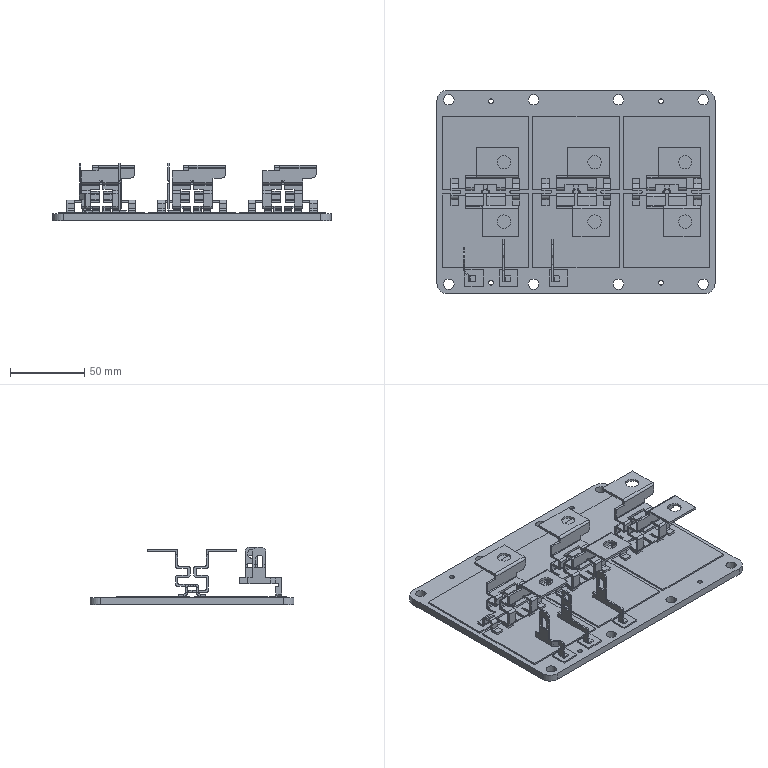Part | SolidWorks | features ReferencePattern 4, LocalLPattern 1 | 10 solids | 1160 faces | box 187 x 137 x 38.97 mm | volume 158216 mm3 | plane 798 | cylinder 362 | commonest cylinder face diameters 1 x136 3 x72 4 x36 1.473 x24 4.473 x24 7 x16